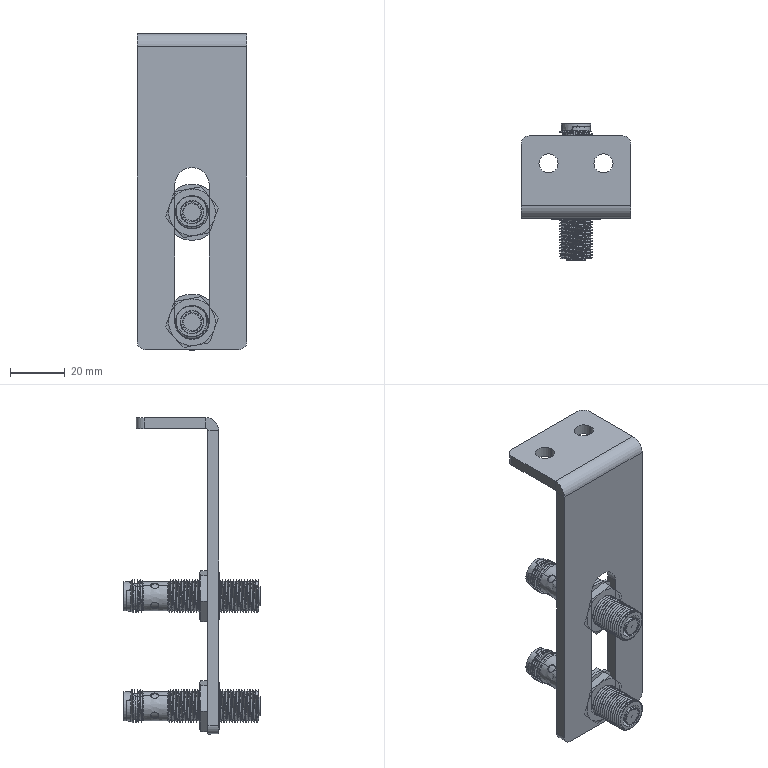Part | SolidWorks | 1 solid | 1331 faces | box 40 x 49.5 x 115.25 mm | volume 18897 mm3 | cylinder 475 | spline 380 | plane 362 | cone 86 | torus 20 | sphere 8 | commonest cylinder face diameters 12 x124 0.2 x96 1 x44 2.031 x28 2 x22 12.93 x22